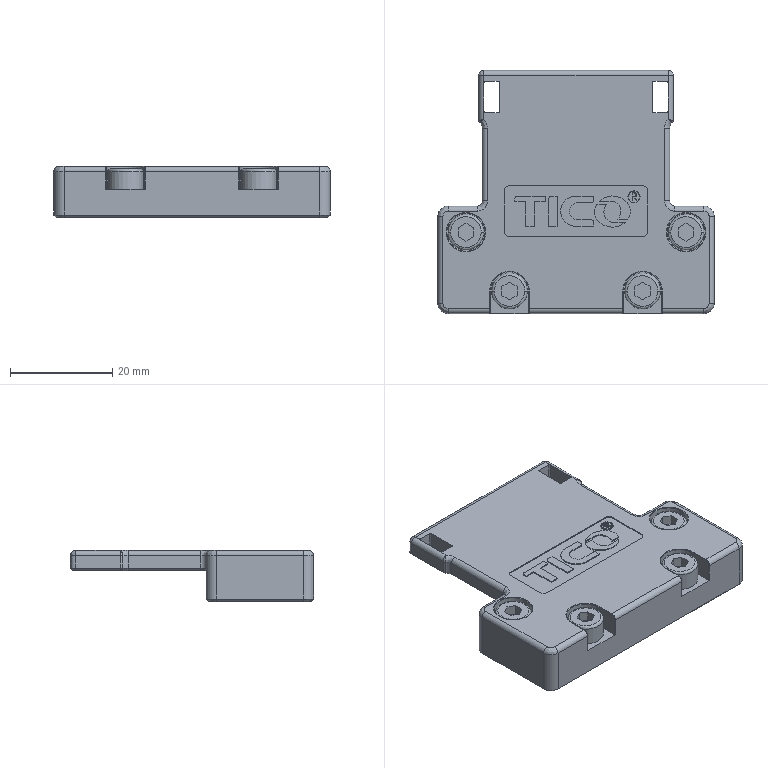Part | SolidWorks | features BaseBody 1 | 1 solid | 265 faces | box 54 x 47.5 x 10 mm | volume 14283 mm3 | plane 126 | cylinder 90 | spline 37 | cone 12 | commonest cylinder face diameters 2 x22 0.2 x8 0.6 x8 4.5 x8 7 x8 4 x6